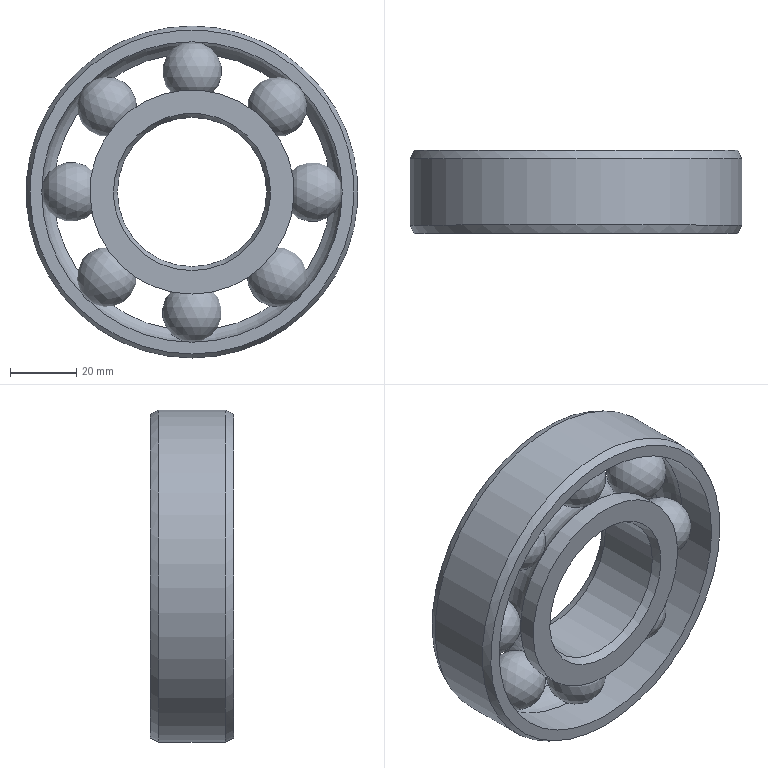Part | NX | features DATUM_CSYS 10, SKETCH 9, SWP104 9, EXTRACT_DATUM_AXIS 8, EXTRACT_DATUM_PLANE 8, EXTRACT_STRING 8, Instance Feature 7, Pattern Feature 1 | 10 solids | 24 faces | box 100 x 25 x 100 mm | volume 93926 mm3 | sphere 8 | cylinder 6 | plane 4 | cone 4 | torus 2 | commonest cylinder face diameters 61.5 x2 45 x1 83.5 x1 90.5 x1 100 x1
STEP:
#1=CARTESIAN_POINT('',(0.,12.5,27.25));
#2=VERTEX_POINT('',#1);
#3=VERTEX_LOOP('',#2);
#4=FACE_BOUND('',#3,.T.);
#5=CARTESIAN_POINT('',(0.,12.5,36.25));
#6=DIRECTION('',(0.,0.,1.));
#7=DIRECTION('',(0.,1.,0.));
#8=AXIS2_PLACEMENT_3D('',#5,#6,#7);
#9=SPHERICAL_SURFACE('',#8,9.);
#10=ADVANCED_FACE('',(#4),#9,.T.);
#11=CLOSED_SHELL('',(#10));
#12=MANIFOLD_SOLID_BREP('',#11);
#13=CARTESIAN_POINT('',(0.,0.,-23.7));
#14=VERTEX_POINT('',#13);
#15=CARTESIAN_POINT('',(0.,0.,0.));
#16=DIRECTION('',(0.,-1.,0.));
#17=DIRECTION('',(0.,0.,-1.));
#18=AXIS2_PLACEMENT_3D('',#15,#16,#17);
#19=CIRCLE('',#18,23.7);
#20=EDGE_CURVE('',#14,#14,#19,.T.);
#21=ORIENTED_EDGE('',*,*,#20,.F.);
#22=EDGE_LOOP('',(#21));
#23=FACE_BOUND('',#22,.T.);
#24=CARTESIAN_POINT('',(0.,0.,-30.75));
#25=VERTEX_POINT('',#24);
#26=CARTESIAN_POINT('',(0.,0.,0.));
#27=DIRECTION('',(0.,-1.,0.));
#28=DIRECTION('',(0.,0.,-1.));
#29=AXIS2_PLACEMENT_3D('',#26,#27,#28);
#30=CIRCLE('',#29,30.75);
#31=EDGE_CURVE('',#25,#25,#30,.T.);
#32=ORIENTED_EDGE('',*,*,#31,.T.);
#33=EDGE_LOOP('',(#32));
#34=FACE_BOUND('',#33,.T.);
#35=CARTESIAN_POINT('',(0.,0.,30.75));
#36=DIRECTION('',(0.,1.,0.));
#37=DIRECTION('',(0.,0.,1.));
#38=AXIS2_PLACEMENT_3D('',#35,#36,#37);
#39=PLANE('',#38);
#40=ADVANCED_FACE('',(#23,#34),#39,.F.);
#41=CARTESIAN_POINT('',(0.,2.5,-22.5));
#42=VERTEX_POINT('',#41);
#43=CARTESIAN_POINT('',(0.,2.5,0.));
#44=DIRECTION('',(0.,-1.,0.));
#45=DIRECTION('',(0.,0.,-1.));
#46=AXIS2_PLACEMENT_3D('',#43,#44,#45);
#47=CIRCLE('',#46,22.5);
#48=EDGE_CURVE('',#42,#42,#47,.T.);
#49=ORIENTED_EDGE('',*,*,#48,.F.);
#50=EDGE_LOOP('',(#49));
#51=FACE_BOUND('',#50,.T.);
#52=ORIENTED_EDGE('',*,*,#20,.T.);
#53=EDGE_LOOP('',(#52));
#54=FACE_BOUND('',#53,.T.);
#55=CARTESIAN_POINT('',(0.,0.,0.));
#56=DIRECTION('',(0.,-1.,0.));
#57=DIRECTION('',(0.,0.,-1.));
#58=AXIS2_PLACEMENT_3D('',#55,#56,#57);
#59=CONICAL_SURFACE('',#58,23.7,0.4475);
#60=ADVANCED_FACE('',(#51,#54),#59,.F.);
#61=CARTESIAN_POINT('',(0.,22.5,-22.5));
#62=VERTEX_POINT('',#61);
#63=CARTESIAN_POINT('',(0.,22.5,0.));
#64=DIRECTION('',(0.,-1.,0.));
#65=DIRECTION('',(0.,0.,-1.));
#66=AXIS2_PLACEMENT_3D('',#63,#64,#65);
#67=CIRCLE('',#66,22.5);
#68=EDGE_CURVE('',#62,#62,#67,.T.);
#69=ORIENTED_EDGE('',*,*,#68,.F.);
#70=EDGE_LOOP('',(#69));
#71=FACE_BOUND('',#70,.T.);
#72=ORIENTED_EDGE('',*,*,#48,.T.);
#73=EDGE_LOOP('',(#72));
#74=FACE_BOUND('',#73,.T.);
#75=CARTESIAN_POINT('',(0.,0.,0.));
#76=DIRECTION('',(0.,-1.,0.));
#77=DIRECTION('',(0.,0.,-1.));
#78=AXIS2_PLACEMENT_3D('',#75,#76,#77);
#79=CYLINDRICAL_SURFACE('',#78,22.5);
#80=ADVANCED_FACE('',(#71,#74),#79,.F.);
#81=CARTESIAN_POINT('',(0.,25.,-23.7));
#82=VERTEX_POINT('',#81);
#83=CARTESIAN_POINT('',(0.,25.,0.));
#84=DIRECTION('',(0.,-1.,0.));
#85=DIRECTION('',(0.,0.,-1.));
#86=AXIS2_PLACEMENT_3D('',#83,#84,#85);
#87=CIRCLE('',#86,23.7);
#88=EDGE_CURVE('',#82,#82,#87,.T.);
#89=ORIENTED_EDGE('',*,*,#88,.F.);
#90=EDGE_LOOP('',(#89));
#91=FACE_BOUND('',#90,.T.);
#92=ORIENTED_EDGE('',*,*,#68,.T.);
#93=EDGE_LOOP('',(#92));
#94=FACE_BOUND('',#93,.T.);
#95=CARTESIAN_POINT('',(0.,22.5,0.));
#96=DIRECTION('',(0.,1.,0.));
#97=DIRECTION('',(0.,0.,1.));
#98=AXIS2_PLACEMENT_3D('',#95,#96,#97);
#99=CONICAL_SURFACE('',#98,22.5,0.4475);
#100=ADVANCED_FACE('',(#91,#94),#99,.F.);
#101=CARTESIAN_POINT('',(0.,25.,-30.75));
#102=VERTEX_POINT('',#101);
#103=CARTESIAN_POINT('',(0.,25.,0.));
#104=DIRECTION('',(0.,-1.,0.));
#105=DIRECTION('',(0.,0.,-1.));
#106=AXIS2_PLACEMENT_3D('',#103,#104,#105);
#107=CIRCLE('',#106,30.75);
#108=EDGE_CURVE('',#102,#102,#107,.T.);
#109=ORIENTED_EDGE('',*,*,#108,.F.);
#110=EDGE_LOOP('',(#109));
#111=FACE_BOUND('',#110,.T.);
#112=ORIENTED_EDGE('',*,*,#88,.T.);
#113=EDGE_LOOP('',(#112));
#114=FACE_BOUND('',#113,.T.);
#115=CARTESIAN_POINT('',(0.,25.,23.7));
#116=DIRECTION('',(0.,-1.,0.));
#117=DIRECTION('',(0.,0.,-1.));
#118=AXIS2_PLACEMENT_3D('',#115,#116,#117);
#119=PLANE('',#118);
#120=ADVANCED_FACE('',(#111,#114),#119,.F.);
#121=CARTESIAN_POINT('',(0.,19.624,-30.75));
#122=VERTEX_POINT('',#121);
#123=CARTESIAN_POINT('',(0.,19.624,0.));
#124=DIRECTION('',(0.,-1.,0.));
#125=DIRECTION('',(0.,0.,-1.));
#126=AXIS2_PLACEMENT_3D('',#123,#124,#125);
#127=CIRCLE('',#126,30.75);
#128=EDGE_CURVE('',#122,#122,#127,.T.);
#129=ORIENTED_EDGE('',*,*,#128,.F.);
#130=EDGE_LOOP('',(#129));
#131=FACE_BOUND('',#130,.T.);
#132=ORIENTED_EDGE('',*,*,#108,.T.);
#133=EDGE_LOOP('',(#132));
#134=FACE_BOUND('',#133,.T.);
#135=CARTESIAN_POINT('',(0.,0.,0.));
#136=DIRECTION('',(0.,-1.,0.));
#137=DIRECTION('',(0.,0.,-1.));
#138=AXIS2_PLACEMENT_3D('',#135,#136,#137);
#139=CYLINDRICAL_SURFACE('',#138,30.75);
#140=ADVANCED_FACE('',(#131,#134),#139,.T.);
#141=CARTESIAN_POINT('',(0.,5.376,-30.75));
#142=VERTEX_POINT('',#141);
#143=CARTESIAN_POINT('',(0.,5.376,0.));
#144=DIRECTION('',(0.,-1.,0.));
#145=DIRECTION('',(0.,0.,-1.));
#146=AXIS2_PLACEMENT_3D('',#143,#144,#145);
#147=CIRCLE('',#146,30.75);
#148=EDGE_CURVE('',#142,#142,#147,.T.);
#149=ORIENTED_EDGE('',*,*,#148,.F.);
#150=EDGE_LOOP('',(#149));
#151=FACE_BOUND('',#150,.T.);
#152=ORIENTED_EDGE('',*,*,#128,.T.);
#153=EDGE_LOOP('',(#152));
#154=FACE_BOUND('',#153,.T.);
#155=CARTESIAN_POINT('',(0.,12.5,0.));
#156=DIRECTION('',(0.,-1.,0.));
#157=DIRECTION('',(0.,0.,-1.));
#158=AXIS2_PLACEMENT_3D('',#155,#156,#157);
#159=TOROIDAL_SURFACE('',#158,36.25,9.);
#160=ADVANCED_FACE('',(#151,#154),#159,.F.);
#161=ORIENTED_EDGE('',*,*,#31,.F.);
#162=EDGE_LOOP('',(#161));
#163=FACE_BOUND('',#162,.T.);
#164=ORIENTED_EDGE('',*,*,#148,.T.);
#165=EDGE_LOOP('',(#164));
#166=FACE_BOUND('',#165,.T.);
#167=CARTESIAN_POINT('',(0.,0.,0.));
#168=DIRECTION('',(0.,-1.,0.));
#169=DIRECTION('',(0.,0.,-1.));
#170=AXIS2_PLACEMENT_3D('',#167,#168,#169);
#171=CYLINDRICAL_SURFACE('',#170,30.75);
#172=ADVANCED_FACE('',(#163,#166),#171,.T.);
#173=CLOSED_SHELL('',(#40,#60,#80,#100,#120,#140,#160,#172));
#174=MANIFOLD_SOLID_BREP('',#173);
#175=CARTESIAN_POINT('',(-19.269,12.5,19.269));
#176=VERTEX_POINT('',#175);
#177=VERTEX_LOOP('',#176);
#178=FACE_BOUND('',#177,.T.);
#179=CARTESIAN_POINT('',(-25.633,12.5,25.633));
#180=DIRECTION('',(-0.7071,0.,0.7071));
#181=DIRECTION('',(0.,1.,0.));
#182=AXIS2_PLACEMENT_3D('',#179,#180,#181);
#183=SPHERICAL_SURFACE('',#182,9.);
#184=ADVANCED_FACE('',(#178),#183,.T.);
#185=CLOSED_SHELL('',(#184));
#186=MANIFOLD_SOLID_BREP('',#185);
#187=CARTESIAN_POINT('',(27.25,12.5,0.));
#188=VERTEX_POINT('',#187);
#189=VERTEX_LOOP('',#188);
#190=FACE_BOUND('',#189,.T.);
#191=CARTESIAN_POINT('',(36.25,12.5,0.));
#192=DIRECTION('',(1.,0.,0.));
#193=DIRECTION('',(0.,1.,0.));
#194=AXIS2_PLACEMENT_3D('',#191,#192,#193);
#195=SPHERICAL_SURFACE('',#194,9.);
#196=ADVANCED_FACE('',(#190),#195,.T.);
#197=CLOSED_SHELL('',(#196));
#198=MANIFOLD_SOLID_BREP('',#197);
#199=CARTESIAN_POINT('',(-27.25,12.5,0.));
#200=VERTEX_POINT('',#199);
#201=VERTEX_LOOP('',#200);
#202=FACE_BOUND('',#201,.T.);
#203=CARTESIAN_POINT('',(-36.25,12.5,0.));
#204=DIRECTION('',(-1.,0.,0.));
#205=DIRECTION('',(0.,1.,0.));
#206=AXIS2_PLACEMENT_3D('',#203,#204,#205);
#207=SPHERICAL_SURFACE('',#206,9.);
#208=ADVANCED_FACE('',(#202),#207,.T.);
#209=CLOSED_SHELL('',(#208));
#210=MANIFOLD_SOLID_BREP('',#209);
#211=CARTESIAN_POINT('',(19.269,12.5,19.269));
#212=VERTEX_POINT('',#211);
#213=VERTEX_LOOP('',#212);
#214=FACE_BOUND('',#213,.T.);
#215=CARTESIAN_POINT('',(25.633,12.5,25.633));
#216=DIRECTION('',(0.7071,0.,0.7071));
#217=DIRECTION('',(0.,1.,0.));
#218=AXIS2_PLACEMENT_3D('',#215,#216,#217);
#219=SPHERICAL_SURFACE('',#218,9.);
#220=ADVANCED_FACE('',(#214),#219,.T.);
#221=CLOSED_SHELL('',(#220));
#222=MANIFOLD_SOLID_BREP('',#221);
#223=CARTESIAN_POINT('',(-19.269,12.5,-19.269));
#224=VERTEX_POINT('',#223);
#225=VERTEX_LOOP('',#224);
#226=FACE_BOUND('',#225,.T.);
#227=CARTESIAN_POINT('',(-25.633,12.5,-25.633));
#228=DIRECTION('',(-0.7071,0.,-0.7071));
#229=DIRECTION('',(0.,1.,0.));
#230=AXIS2_PLACEMENT_3D('',#227,#228,#229);
#231=SPHERICAL_SURFACE('',#230,9.);
#232=ADVANCED_FACE('',(#226),#231,.T.);
#233=CLOSED_SHELL('',(#232));
#234=MANIFOLD_SOLID_BREP('',#233);
#235=CARTESIAN_POINT('',(19.269,12.5,-19.269));
#236=VERTEX_POINT('',#235);
#237=VERTEX_LOOP('',#236);
#238=FACE_BOUND('',#237,.T.);
#239=CARTESIAN_POINT('',(25.633,12.5,-25.633));
#240=DIRECTION('',(0.7071,0.,-0.7071));
#241=DIRECTION('',(0.,1.,0.));
#242=AXIS2_PLACEMENT_3D('',#239,#240,#241);
#243=SPHERICAL_SURFACE('',#242,9.);
#244=ADVANCED_FACE('',(#238),#243,.T.);
#245=CLOSED_SHELL('',(#244));
#246=MANIFOLD_SOLID_BREP('',#245);
#247=CARTESIAN_POINT('',(0.,0.,-45.25));
#248=VERTEX_POINT('',#247);
#249=CARTESIAN_POINT('',(0.,0.,0.));
#250=DIRECTION('',(0.,-1.,0.));
#251=DIRECTION('',(0.,0.,-1.));
#252=AXIS2_PLACEMENT_3D('',#249,#250,#251);
#253=CIRCLE('',#252,45.25);
#254=EDGE_CURVE('',#248,#248,#253,.T.);
#255=ORIENTED_EDGE('',*,*,#254,.F.);
#256=EDGE_LOOP('',(#255));
#257=FACE_BOUND('',#256,.T.);
#258=CARTESIAN_POINT('',(0.,0.,-48.8));
#259=VERTEX_POINT('',#258);
#260=CARTESIAN_POINT('',(0.,0.,0.));
#261=DIRECTION('',(0.,-1.,0.));
#262=DIRECTION('',(0.,0.,-1.));
#263=AXIS2_PLACEMENT_3D('',#260,#261,#262);
#264=CIRCLE('',#263,48.8);
#265=EDGE_CURVE('',#259,#259,#264,.T.);
#266=ORIENTED_EDGE('',*,*,#265,.T.);
#267=EDGE_LOOP('',(#266));
#268=FACE_BOUND('',#267,.T.);
#269=CARTESIAN_POINT('',(0.,0.,48.8));
#270=DIRECTION('',(0.,1.,0.));
#271=DIRECTION('',(0.,0.,1.));
#272=AXIS2_PLACEMENT_3D('',#269,#270,#271);
#273=PLANE('',#272);
#274=ADVANCED_FACE('',(#257,#268),#273,.F.);
#275=CARTESIAN_POINT('',(0.,12.5,-45.25));
#276=VERTEX_POINT('',#275);
#277=CARTESIAN_POINT('',(0.,12.5,0.));
#278=DIRECTION('',(0.,-1.,0.));
#279=DIRECTION('',(0.,0.,-1.));
#280=AXIS2_PLACEMENT_3D('',#277,#278,#279);
#281=CIRCLE('',#280,45.25);
#282=EDGE_CURVE('',#276,#276,#281,.T.);
#283=ORIENTED_EDGE('',*,*,#282,.F.);
#284=EDGE_LOOP('',(#283));
#285=FACE_BOUND('',#284,.T.);
#286=ORIENTED_EDGE('',*,*,#254,.T.);
#287=EDGE_LOOP('',(#286));
#288=FACE_BOUND('',#287,.T.);
#289=CARTESIAN_POINT('',(0.,0.,0.));
#290=DIRECTION('',(0.,-1.,0.));
#291=DIRECTION('',(0.,0.,-1.));
#292=AXIS2_PLACEMENT_3D('',#289,#290,#291);
#293=CYLINDRICAL_SURFACE('',#292,45.25);
#294=ADVANCED_FACE('',(#285,#288),#293,.F.);
#295=CARTESIAN_POINT('',(0.,19.624,-41.75));
#296=VERTEX_POINT('',#295);
#297=CARTESIAN_POINT('',(0.,19.624,0.));
#298=DIRECTION('',(0.,-1.,0.));
#299=DIRECTION('',(0.,0.,-1.));
#300=AXIS2_PLACEMENT_3D('',#297,#298,#299);
#301=CIRCLE('',#300,41.75);
#302=EDGE_CURVE('',#296,#296,#301,.T.);
#303=ORIENTED_EDGE('',*,*,#302,.F.);
#304=EDGE_LOOP('',(#303));
#305=FACE_BOUND('',#304,.T.);
#306=ORIENTED_EDGE('',*,*,#282,.T.);
#307=EDGE_LOOP('',(#306));
#308=FACE_BOUND('',#307,.T.);
#309=CARTESIAN_POINT('',(0.,12.5,0.));
#310=DIRECTION('',(0.,-1.,0.));
#311=DIRECTION('',(0.,0.,-1.));
#312=AXIS2_PLACEMENT_3D('',#309,#310,#311);
#313=TOROIDAL_SURFACE('',#312,36.25,9.);
#314=ADVANCED_FACE('',(#305,#308),#313,.F.);
#315=CARTESIAN_POINT('',(0.,25.,-41.75));
#316=VERTEX_POINT('',#315);
#317=CARTESIAN_POINT('',(0.,25.,0.));
#318=DIRECTION('',(0.,-1.,0.));
#319=DIRECTION('',(0.,0.,-1.));
#320=AXIS2_PLACEMENT_3D('',#317,#318,#319);
#321=CIRCLE('',#320,41.75);
#322=EDGE_CURVE('',#316,#316,#321,.T.);
#323=ORIENTED_EDGE('',*,*,#322,.F.);
#324=EDGE_LOOP('',(#323));
#325=FACE_BOUND('',#324,.T.);
#326=ORIENTED_EDGE('',*,*,#302,.T.);
#327=EDGE_LOOP('',(#326));
#328=FACE_BOUND('',#327,.T.);
#329=CARTESIAN_POINT('',(0.,0.,0.));
#330=DIRECTION('',(0.,-1.,0.));
#331=DIRECTION('',(0.,0.,-1.));
#332=AXIS2_PLACEMENT_3D('',#329,#330,#331);
#333=CYLINDRICAL_SURFACE('',#332,41.75);
#334=ADVANCED_FACE('',(#325,#328),#333,.F.);
#335=CARTESIAN_POINT('',(0.,25.,-48.8));
#336=VERTEX_POINT('',#335);
#337=CARTESIAN_POINT('',(0.,25.,0.));
#338=DIRECTION('',(0.,-1.,0.));
#339=DIRECTION('',(0.,0.,-1.));
#340=AXIS2_PLACEMENT_3D('',#337,#338,#339);
#341=CIRCLE('',#340,48.8);
#342=EDGE_CURVE('',#336,#336,#341,.T.);
#343=ORIENTED_EDGE('',*,*,#342,.F.);
#344=EDGE_LOOP('',(#343));
#345=FACE_BOUND('',#344,.T.);
#346=ORIENTED_EDGE('',*,*,#322,.T.);
#347=EDGE_LOOP('',(#346));
#348=FACE_BOUND('',#347,.T.);
#349=CARTESIAN_POINT('',(0.,25.,41.75));
#350=DIRECTION('',(0.,-1.,0.));
#351=DIRECTION('',(0.,0.,-1.));
#352=AXIS2_PLACEMENT_3D('',#349,#350,#351);
#353=PLANE('',#352);
#354=ADVANCED_FACE('',(#345,#348),#353,.F.);
#355=CARTESIAN_POINT('',(0.,22.5,-50.));
#356=VERTEX_POINT('',#355);
#357=CARTESIAN_POINT('',(0.,22.5,0.));
#358=DIRECTION('',(0.,-1.,0.));
#359=DIRECTION('',(0.,0.,-1.));
#360=AXIS2_PLACEMENT_3D('',#357,#358,#359);
#361=CIRCLE('',#360,50.);
#362=EDGE_CURVE('',#356,#356,#361,.T.);
#363=ORIENTED_EDGE('',*,*,#362,.F.);
#364=EDGE_LOOP('',(#363));
#365=FACE_BOUND('',#364,.T.);
#366=ORIENTED_EDGE('',*,*,#342,.T.);
#367=EDGE_LOOP('',(#366));
#368=FACE_BOUND('',#367,.T.);
#369=CARTESIAN_POINT('',(0.,25.,0.));
#370=DIRECTION('',(0.,-1.,0.));
#371=DIRECTION('',(0.,0.,-1.));
#372=AXIS2_PLACEMENT_3D('',#369,#370,#371);
#373=CONICAL_SURFACE('',#372,48.8,0.4475);
#374=ADVANCED_FACE('',(#365,#368),#373,.T.);
#375=CARTESIAN_POINT('',(0.,2.5,-50.));
#376=VERTEX_POINT('',#375);
#377=CARTESIAN_POINT('',(0.,2.5,0.));
#378=DIRECTION('',(0.,-1.,0.));
#379=DIRECTION('',(0.,0.,-1.));
#380=AXIS2_PLACEMENT_3D('',#377,#378,#379);
#381=CIRCLE('',#380,50.);
#382=EDGE_CURVE('',#376,#376,#381,.T.);
#383=ORIENTED_EDGE('',*,*,#382,.F.);
#384=EDGE_LOOP('',(#383));
#385=FACE_BOUND('',#384,.T.);
#386=ORIENTED_EDGE('',*,*,#362,.T.);
#387=EDGE_LOOP('',(#386));
#388=FACE_BOUND('',#387,.T.);
#389=CARTESIAN_POINT('',(0.,0.,0.));
#390=DIRECTION('',(0.,-1.,0.));
#391=DIRECTION('',(0.,0.,-1.));
#392=AXIS2_PLACEMENT_3D('',#389,#390,#391);
#393=CYLINDRICAL_SURFACE('',#392,50.);
#394=ADVANCED_FACE('',(#385,#388),#393,.T.);
#395=ORIENTED_EDGE('',*,*,#265,.F.);
#396=EDGE_LOOP('',(#395));
#397=FACE_BOUND('',#396,.T.);
#398=ORIENTED_EDGE('',*,*,#382,.T.);
#399=EDGE_LOOP('',(#398));
#400=FACE_BOUND('',#399,.T.);
#401=CARTESIAN_POINT('',(0.,2.5,0.));
#402=DIRECTION('',(0.,1.,0.));
#403=DIRECTION('',(0.,0.,1.));
#404=AXIS2_PLACEMENT_3D('',#401,#402,#403);
#405=CONICAL_SURFACE('',#404,50.,0.4475);
#406=ADVANCED_FACE('',(#397,#400),#405,.T.);
#407=CLOSED_SHELL('',(#274,#294,#314,#334,#354,#374,#394,#406));
#408=MANIFOLD_SOLID_BREP('',#407);
#409=CARTESIAN_POINT('',(0.,12.5,-27.25));
#410=VERTEX_POINT('',#409);
#411=VERTEX_LOOP('',#410);
#412=FACE_BOUND('',#411,.T.);
#413=CARTESIAN_POINT('',(0.,12.5,-36.25));
#414=DIRECTION('',(0.,0.,-1.));
#415=DIRECTION('',(0.,1.,0.));
#416=AXIS2_PLACEMENT_3D('',#413,#414,#415);
#417=SPHERICAL_SURFACE('',#416,9.);
#418=ADVANCED_FACE('',(#412),#417,.T.);
#419=CLOSED_SHELL('',(#418));
#420=MANIFOLD_SOLID_BREP('',#419);
#421=(LENGTH_UNIT()NAMED_UNIT(*)SI_UNIT(.MILLI.,.METRE.));
#422=UNCERTAINTY_MEASURE_WITH_UNIT(LENGTH_MEASURE(0.00001),#421,'','');
#423=(NAMED_UNIT(*)PLANE_ANGLE_UNIT()SI_UNIT($,.RADIAN.));
#424=(NAMED_UNIT(*)SI_UNIT($,.STERADIAN.)SOLID_ANGLE_UNIT());
#425=(GEOMETRIC_REPRESENTATION_CONTEXT(3)GLOBAL_UNCERTAINTY_ASSIGNED_CONTEXT((#422))GLOBAL_UNIT_ASSIGNED_CONTEXT((#421,#423,#424))REPRESENTATION_CONTEXT('',''));
#426=ADVANCED_BREP_SHAPE_REPRESENTATION('',(#12,#174,#186,#198,#210,#222,#234,#246,#408,#420),#425);